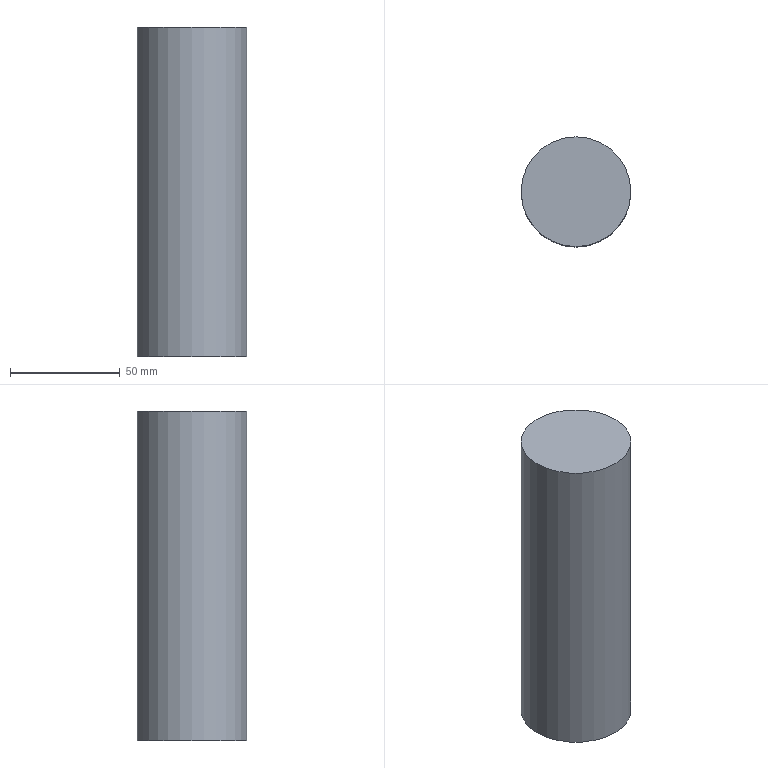Part | NX | features 模具.stp<1>[109] 2 | 1 solid | 11 faces | box 50 x 50 x 150 mm | volume 291726 mm3 | plane 6 | cylinder 4 | cone 1 | commonest cylinder face diameters 10.5 x1 11.7 x1 12 x1 50 x1
STEP:
#1=CARTESIAN_POINT('',(-70.,-100.,-217.505));
#2=VERTEX_POINT('',#1);
#3=VERTEX_LOOP('',#2);
#4=FACE_BOUND('',#3,.T.);
#5=CARTESIAN_POINT('',(-70.,-94.75,-220.536));
#6=VERTEX_POINT('',#5);
#7=CARTESIAN_POINT('',(-70.,-100.,-220.536));
#8=DIRECTION('',(0.,0.,-1.));
#9=DIRECTION('',(0.,1.,0.));
#10=AXIS2_PLACEMENT_3D('',#7,#8,#9);
#11=CIRCLE('',#10,5.25);
#12=EDGE_CURVE('',#6,#6,#11,.T.);
#13=ORIENTED_EDGE('',*,*,#12,.T.);
#14=EDGE_LOOP('',(#13));
#15=FACE_BOUND('',#14,.T.);
#16=CARTESIAN_POINT('',(-70.,-100.,-218.505));
#17=DIRECTION('',(0.,0.,-1.));
#18=DIRECTION('',(0.,1.,0.));
#19=AXIS2_PLACEMENT_3D('',#16,#17,#18);
#20=CONICAL_SURFACE('',#19,1.732,1.047);
#21=ADVANCED_FACE('',(#4,#15),#20,.F.);
#22=CARTESIAN_POINT('',(-70.,-94.75,-227.5));
#23=VERTEX_POINT('',#22);
#24=CARTESIAN_POINT('',(-70.,-94.15,-227.5));
#25=VERTEX_POINT('',#24);
#26=CARTESIAN_POINT('',(-70.,-100.,-227.5));
#27=DIRECTION('',(0.,1.,0.));
#28=VECTOR('',#27,1000.);
#29=LINE('',#26,#28);
#30=EDGE_CURVE('',#23,#25,#29,.T.);
#31=ORIENTED_EDGE('',*,*,#30,.T.);
#32=CARTESIAN_POINT('',(-64.15,-100.,-227.5));
#33=VERTEX_POINT('',#32);
#34=CARTESIAN_POINT('',(-70.,-100.,-227.5));
#35=DIRECTION('',(0.,0.,1.));
#36=DIRECTION('',(0.,1.,0.));
#37=AXIS2_PLACEMENT_3D('',#34,#35,#36);
#38=CIRCLE('',#37,5.85);
#39=EDGE_CURVE('',#25,#33,#38,.T.);
#40=ORIENTED_EDGE('',*,*,#39,.T.);
#41=CARTESIAN_POINT('',(-64.75,-100.,-227.5));
#42=VERTEX_POINT('',#41);
#43=CARTESIAN_POINT('',(-70.,-100.,-227.5));
#44=DIRECTION('',(-1.,0.,0.));
#45=VECTOR('',#44,1000.);
#46=LINE('',#43,#45);
#47=EDGE_CURVE('',#33,#42,#46,.T.);
#48=ORIENTED_EDGE('',*,*,#47,.T.);
#49=CARTESIAN_POINT('',(-70.,-100.,-227.5));
#50=DIRECTION('',(0.,0.,-1.));
#51=DIRECTION('',(0.,-1.,0.));
#52=AXIS2_PLACEMENT_3D('',#49,#50,#51);
#53=CIRCLE('',#52,5.25);
#54=EDGE_CURVE('',#42,#23,#53,.T.);
#55=ORIENTED_EDGE('',*,*,#54,.T.);
#56=EDGE_LOOP('',(#31,#40,#48,#55));
#57=FACE_BOUND('',#56,.T.);
#58=CARTESIAN_POINT('',(-70.,-100.,-227.5));
#59=DIRECTION('',(0.,0.,1.));
#60=DIRECTION('',(0.,-1.,0.));
#61=AXIS2_PLACEMENT_3D('',#58,#59,#60);
#62=PLANE('',#61);
#63=ADVANCED_FACE('',(#57),#62,.T.);
#64=CARTESIAN_POINT('',(-64.75,-100.,-226.5));
#65=VERTEX_POINT('',#64);
#66=CARTESIAN_POINT('',(-70.,-94.75,-226.5));
#67=VERTEX_POINT('',#66);
#68=CARTESIAN_POINT('',(-70.,-100.,-226.5));
#69=DIRECTION('',(0.,0.,-1.));
#70=DIRECTION('',(0.,-1.,0.));
#71=AXIS2_PLACEMENT_3D('',#68,#69,#70);
#72=CIRCLE('',#71,5.25);
#73=EDGE_CURVE('',#65,#67,#72,.T.);
#74=ORIENTED_EDGE('',*,*,#73,.F.);
#75=CARTESIAN_POINT('',(-64.,-100.,-226.5));
#76=VERTEX_POINT('',#75);
#77=CARTESIAN_POINT('',(-64.,-100.,-226.5));
#78=DIRECTION('',(1.,0.,0.));
#79=VECTOR('',#78,1000.);
#80=LINE('',#77,#79);
#81=EDGE_CURVE('',#65,#76,#80,.T.);
#82=ORIENTED_EDGE('',*,*,#81,.T.);
#83=CARTESIAN_POINT('',(-70.,-94.,-226.5));
#84=VERTEX_POINT('',#83);
#85=CARTESIAN_POINT('',(-70.,-100.,-226.5));
#86=DIRECTION('',(0.,0.,1.));
#87=DIRECTION('',(0.,1.,0.));
#88=AXIS2_PLACEMENT_3D('',#85,#86,#87);
#89=CIRCLE('',#88,6.);
#90=EDGE_CURVE('',#84,#76,#89,.T.);
#91=ORIENTED_EDGE('',*,*,#90,.F.);
#92=CARTESIAN_POINT('',(-70.,-94.,-226.5));
#93=DIRECTION('',(0.,-1.,0.));
#94=VECTOR('',#93,1000.);
#95=LINE('',#92,#94);
#96=EDGE_CURVE('',#84,#67,#95,.T.);
#97=ORIENTED_EDGE('',*,*,#96,.T.);
#98=EDGE_LOOP('',(#74,#82,#91,#97));
#99=FACE_BOUND('',#98,.T.);
#100=CARTESIAN_POINT('',(-70.,-100.,-226.5));
#101=DIRECTION('',(0.,0.,1.));
#102=DIRECTION('',(0.,-1.,0.));
#103=AXIS2_PLACEMENT_3D('',#100,#101,#102);
#104=PLANE('',#103);
#105=ADVANCED_FACE('',(#99),#104,.F.);
#106=CARTESIAN_POINT('',(-64.75,-100.,-250.5));
#107=VERTEX_POINT('',#106);
#108=CARTESIAN_POINT('',(-70.,-100.,-250.5));
#109=DIRECTION('',(0.,0.,1.));
#110=DIRECTION('',(1.,0.,0.));
#111=AXIS2_PLACEMENT_3D('',#108,#109,#110);
#112=CIRCLE('',#111,5.25);
#113=EDGE_CURVE('',#107,#107,#112,.T.);
#114=ORIENTED_EDGE('',*,*,#113,.F.);
#115=EDGE_LOOP('',(#114));
#116=FACE_BOUND('',#115,.T.);
#117=ORIENTED_EDGE('',*,*,#12,.F.);
#118=EDGE_LOOP('',(#117));
#119=FACE_BOUND('',#118,.T.);
#120=CARTESIAN_POINT('',(-70.,-94.75,-220.536));
#121=DIRECTION('',(0.,0.,1.));
#122=VECTOR('',#121,1000.);
#123=LINE('',#120,#122);
#124=EDGE_CURVE('',#23,#67,#123,.T.);
#125=ORIENTED_EDGE('',*,*,#124,.F.);
#126=ORIENTED_EDGE('',*,*,#54,.F.);
#127=CARTESIAN_POINT('',(-64.75,-100.,-220.536));
#128=DIRECTION('',(0.,0.,-1.));
#129=VECTOR('',#128,1000.);
#130=LINE('',#127,#129);
#131=EDGE_CURVE('',#65,#42,#130,.T.);
#132=ORIENTED_EDGE('',*,*,#131,.F.);
#133=ORIENTED_EDGE('',*,*,#73,.T.);
#134=EDGE_LOOP('',(#125,#126,#132,#133));
#135=FACE_BOUND('',#134,.T.);
#136=CARTESIAN_POINT('',(-70.,-100.,-220.536));
#137=DIRECTION('',(0.,0.,-1.));
#138=DIRECTION('',(0.,1.,0.));
#139=AXIS2_PLACEMENT_3D('',#136,#137,#138);
#140=CYLINDRICAL_SURFACE('',#139,5.25);
#141=ADVANCED_FACE('',(#116,#119,#135),#140,.F.);
#142=CARTESIAN_POINT('',(-64.15,-100.,-250.5));
#143=VERTEX_POINT('',#142);
#144=CARTESIAN_POINT('',(-64.,-100.,-250.5));
#145=VERTEX_POINT('',#144);
#146=CARTESIAN_POINT('',(-70.,-100.,-250.5));
#147=DIRECTION('',(1.,0.,0.));
#148=VECTOR('',#147,1000.);
#149=LINE('',#146,#148);
#150=EDGE_CURVE('',#143,#145,#149,.T.);
#151=ORIENTED_EDGE('',*,*,#150,.T.);
#152=CARTESIAN_POINT('',(-64.,-100.,-226.5));
#153=DIRECTION('',(0.,0.,1.));
#154=VECTOR('',#153,1000.);
#155=LINE('',#152,#154);
#156=EDGE_CURVE('',#145,#76,#155,.T.);
#157=ORIENTED_EDGE('',*,*,#156,.T.);
#158=ORIENTED_EDGE('',*,*,#81,.F.);
#159=ORIENTED_EDGE('',*,*,#131,.T.);
#160=ORIENTED_EDGE('',*,*,#47,.F.);
#161=CARTESIAN_POINT('',(-64.15,-100.,-227.5));
#162=DIRECTION('',(0.,0.,1.));
#163=VECTOR('',#162,1000.);
#164=LINE('',#161,#163);
#165=EDGE_CURVE('',#143,#33,#164,.T.);
#166=ORIENTED_EDGE('',*,*,#165,.F.);
#167=EDGE_LOOP('',(#151,#157,#158,#159,#160,#166));
#168=FACE_BOUND('',#167,.T.);
#169=CARTESIAN_POINT('',(-64.,-100.,-226.5));
#170=DIRECTION('',(0.,-1.,0.));
#171=DIRECTION('',(-1.,0.,0.));
#172=AXIS2_PLACEMENT_3D('',#169,#170,#171);
#173=PLANE('',#172);
#174=ADVANCED_FACE('',(#168),#173,.T.);
#175=CARTESIAN_POINT('',(-70.,-94.,-250.5));
#176=VERTEX_POINT('',#175);
#177=CARTESIAN_POINT('',(-70.,-94.15,-250.5));
#178=VERTEX_POINT('',#177);
#179=CARTESIAN_POINT('',(-70.,-100.,-250.5));
#180=DIRECTION('',(0.,-1.,0.));
#181=VECTOR('',#180,1000.);
#182=LINE('',#179,#181);
#183=EDGE_CURVE('',#176,#178,#182,.T.);
#184=ORIENTED_EDGE('',*,*,#183,.T.);
#185=CARTESIAN_POINT('',(-70.,-94.15,-227.5));
#186=DIRECTION('',(0.,0.,-1.));
#187=VECTOR('',#186,1000.);
#188=LINE('',#185,#187);
#189=EDGE_CURVE('',#25,#178,#188,.T.);
#190=ORIENTED_EDGE('',*,*,#189,.F.);
#191=ORIENTED_EDGE('',*,*,#30,.F.);
#192=ORIENTED_EDGE('',*,*,#124,.T.);
#193=ORIENTED_EDGE('',*,*,#96,.F.);
#194=CARTESIAN_POINT('',(-70.,-94.,-226.5));
#195=DIRECTION('',(0.,0.,-1.));
#196=VECTOR('',#195,1000.);
#197=LINE('',#194,#196);
#198=EDGE_CURVE('',#84,#176,#197,.T.);
#199=ORIENTED_EDGE('',*,*,#198,.T.);
#200=EDGE_LOOP('',(#184,#190,#191,#192,#193,#199));
#201=FACE_BOUND('',#200,.T.);
#202=CARTESIAN_POINT('',(-70.,-94.,-226.5));
#203=DIRECTION('',(-1.,0.,0.));
#204=DIRECTION('',(0.,0.,1.));
#205=AXIS2_PLACEMENT_3D('',#202,#203,#204);
#206=PLANE('',#205);
#207=ADVANCED_FACE('',(#201),#206,.T.);
#208=CARTESIAN_POINT('',(-70.,-100.,-250.5));
#209=DIRECTION('',(0.,0.,1.));
#210=DIRECTION('',(1.,0.,0.));
#211=AXIS2_PLACEMENT_3D('',#208,#209,#210);
#212=CIRCLE('',#211,5.85);
#213=EDGE_CURVE('',#178,#143,#212,.T.);
#214=ORIENTED_EDGE('',*,*,#213,.T.);
#215=ORIENTED_EDGE('',*,*,#165,.T.);
#216=ORIENTED_EDGE('',*,*,#39,.F.);
#217=ORIENTED_EDGE('',*,*,#189,.T.);
#218=EDGE_LOOP('',(#214,#215,#216,#217));
#219=FACE_BOUND('',#218,.T.);
#220=CARTESIAN_POINT('',(-70.,-100.,-227.5));
#221=DIRECTION('',(0.,0.,-1.));
#222=DIRECTION('',(0.,1.,0.));
#223=AXIS2_PLACEMENT_3D('',#220,#221,#222);
#224=CYLINDRICAL_SURFACE('',#223,5.85);
#225=ADVANCED_FACE('',(#219),#224,.T.);
#226=ORIENTED_EDGE('',*,*,#198,.F.);
#227=ORIENTED_EDGE('',*,*,#90,.T.);
#228=ORIENTED_EDGE('',*,*,#156,.F.);
#229=CARTESIAN_POINT('',(-70.,-100.,-250.5));
#230=DIRECTION('',(0.,0.,1.));
#231=DIRECTION('',(1.,0.,0.));
#232=AXIS2_PLACEMENT_3D('',#229,#230,#231);
#233=CIRCLE('',#232,6.);
#234=EDGE_CURVE('',#176,#145,#233,.T.);
#235=ORIENTED_EDGE('',*,*,#234,.F.);
#236=EDGE_LOOP('',(#226,#227,#228,#235));
#237=FACE_BOUND('',#236,.T.);
#238=CARTESIAN_POINT('',(-70.,-100.,-226.5));
#239=DIRECTION('',(0.,0.,-1.));
#240=DIRECTION('',(0.,1.,0.));
#241=AXIS2_PLACEMENT_3D('',#238,#239,#240);
#242=CYLINDRICAL_SURFACE('',#241,6.);
#243=ADVANCED_FACE('',(#237),#242,.F.);
#244=CARTESIAN_POINT('',(-70.,-75.,-100.5));
#245=VERTEX_POINT('',#244);
#246=CARTESIAN_POINT('',(-70.,-100.,-100.5));
#247=DIRECTION('',(0.,0.,1.));
#248=DIRECTION('',(0.,1.,0.));
#249=AXIS2_PLACEMENT_3D('',#246,#247,#248);
#250=CIRCLE('',#249,25.);
#251=EDGE_CURVE('',#245,#245,#250,.T.);
#252=ORIENTED_EDGE('',*,*,#251,.T.);
#253=EDGE_LOOP('',(#252));
#254=FACE_BOUND('',#253,.T.);
#255=CARTESIAN_POINT('',(-70.,-100.,-100.5));
#256=DIRECTION('',(0.,0.,1.));
#257=DIRECTION('',(1.,0.,0.));
#258=AXIS2_PLACEMENT_3D('',#255,#256,#257);
#259=PLANE('',#258);
#260=ADVANCED_FACE('',(#254),#259,.T.);
#261=ORIENTED_EDGE('',*,*,#251,.F.);
#262=EDGE_LOOP('',(#261));
#263=FACE_BOUND('',#262,.T.);
#264=CARTESIAN_POINT('',(-70.,-75.,-250.5));
#265=VERTEX_POINT('',#264);
#266=CARTESIAN_POINT('',(-70.,-100.,-250.5));
#267=DIRECTION('',(0.,0.,1.));
#268=DIRECTION('',(0.,1.,0.));
#269=AXIS2_PLACEMENT_3D('',#266,#267,#268);
#270=CIRCLE('',#269,25.);
#271=EDGE_CURVE('',#265,#265,#270,.T.);
#272=ORIENTED_EDGE('',*,*,#271,.T.);
#273=EDGE_LOOP('',(#272));
#274=FACE_BOUND('',#273,.T.);
#275=CARTESIAN_POINT('',(-70.,-100.,-250.5));
#276=DIRECTION('',(0.,0.,1.));
#277=DIRECTION('',(1.,0.,0.));
#278=AXIS2_PLACEMENT_3D('',#275,#276,#277);
#279=CYLINDRICAL_SURFACE('',#278,25.);
#280=ADVANCED_FACE('',(#263,#274),#279,.T.);
#281=ORIENTED_EDGE('',*,*,#183,.F.);
#282=ORIENTED_EDGE('',*,*,#234,.T.);
#283=ORIENTED_EDGE('',*,*,#150,.F.);
#284=ORIENTED_EDGE('',*,*,#213,.F.);
#285=EDGE_LOOP('',(#281,#282,#283,#284));
#286=FACE_BOUND('',#285,.T.);
#287=ORIENTED_EDGE('',*,*,#113,.T.);
#288=EDGE_LOOP('',(#287));
#289=FACE_BOUND('',#288,.T.);
#290=ORIENTED_EDGE('',*,*,#271,.F.);
#291=EDGE_LOOP('',(#290));
#292=FACE_BOUND('',#291,.T.);
#293=CARTESIAN_POINT('',(-70.,-100.,-250.5));
#294=DIRECTION('',(0.,0.,1.));
#295=DIRECTION('',(1.,0.,0.));
#296=AXIS2_PLACEMENT_3D('',#293,#294,#295);
#297=PLANE('',#296);
#298=ADVANCED_FACE('',(#286,#289,#292),#297,.F.);
#299=CLOSED_SHELL('',(#21,#63,#105,#141,#174,#207,#225,#243,#260,#280,#298));
#300=MANIFOLD_SOLID_BREP('',#299);
#301=(LENGTH_UNIT()NAMED_UNIT(*)SI_UNIT(.MILLI.,.METRE.));
#302=UNCERTAINTY_MEASURE_WITH_UNIT(LENGTH_MEASURE(0.00001),#301,'','');
#303=(NAMED_UNIT(*)PLANE_ANGLE_UNIT()SI_UNIT($,.RADIAN.));
#304=(NAMED_UNIT(*)SI_UNIT($,.STERADIAN.)SOLID_ANGLE_UNIT());
#305=(GEOMETRIC_REPRESENTATION_CONTEXT(3)GLOBAL_UNCERTAINTY_ASSIGNED_CONTEXT((#302))GLOBAL_UNIT_ASSIGNED_CONTEXT((#301,#303,#304))REPRESENTATION_CONTEXT('',''));
#306=ADVANCED_BREP_SHAPE_REPRESENTATION('',(#300),#305);